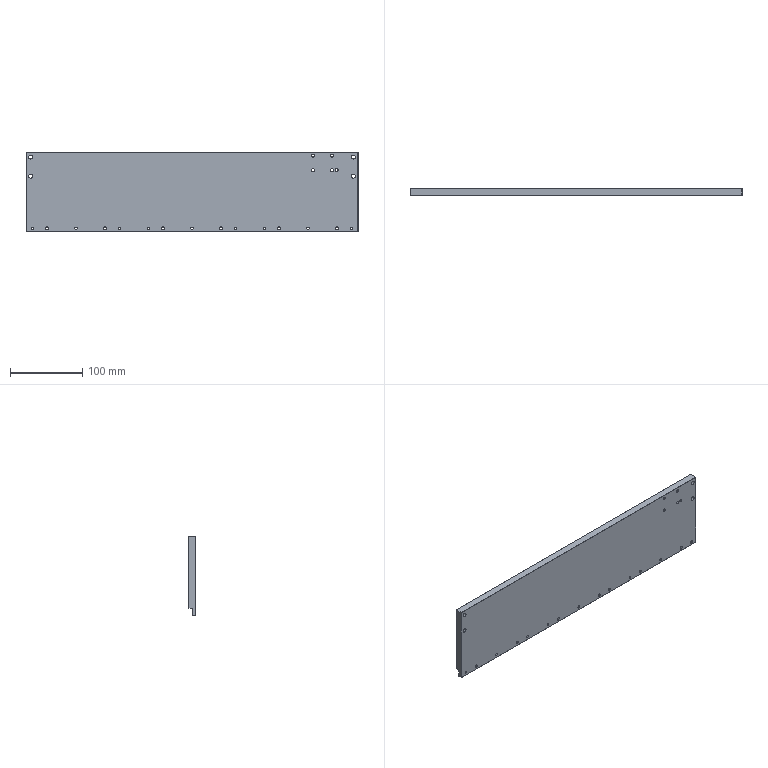Part | NX | 1 solid | 118 faces | box 458 x 10 x 110 mm | volume 475499 mm3 | cone 48 | cylinder 48 | plane 22 | commonest cylinder face diameters 3.3 x18 4 x14 4.2 x8 5.5 x8